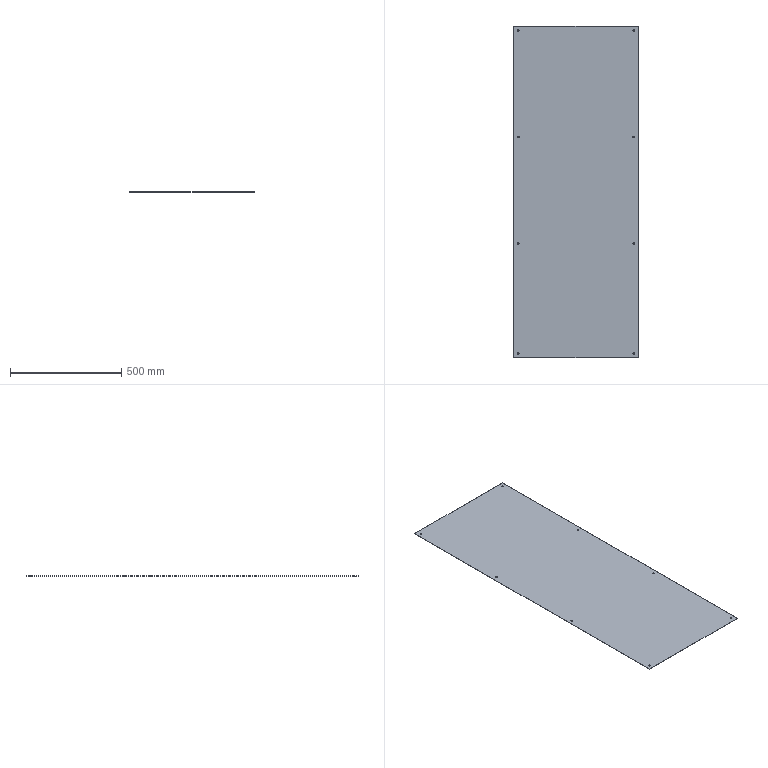Part | SolidWorks | features FlatPattern 1, HoleWzd 1, SMBaseFlange 1, SheetMetal 1 | 1 solid | 22 faces | box 560 x 1495 x 1.2 mm | volume 1004271 mm3 | cylinder 16 | plane 6 | commonest cylinder face diameters 7 x16
STEP:
#1=CARTESIAN_POINT('',(16.5,-1475.,0.));
#2=VERTEX_POINT('',#1);
#3=CARTESIAN_POINT('',(23.5,-1475.,0.));
#4=VERTEX_POINT('',#3);
#5=CARTESIAN_POINT('',(20.,-1475.,0.));
#6=DIRECTION('',(0.,0.,1.));
#7=DIRECTION('',(1.,0.,0.));
#8=AXIS2_PLACEMENT_3D('',#5,#6,#7);
#9=CIRCLE('',#8,3.5);
#10=EDGE_CURVE('',#2,#4,#9,.T.);
#11=ORIENTED_EDGE('',*,*,#10,.F.);
#12=CARTESIAN_POINT('',(16.5,-1475.,1.2));
#13=VERTEX_POINT('',#12);
#14=CARTESIAN_POINT('',(16.5,-1475.,1.2));
#15=DIRECTION('',(0.,0.,1.));
#16=VECTOR('',#15,1000.);
#17=LINE('',#14,#16);
#18=EDGE_CURVE('',#2,#13,#17,.T.);
#19=ORIENTED_EDGE('',*,*,#18,.T.);
#20=CARTESIAN_POINT('',(23.5,-1475.,1.2));
#21=VERTEX_POINT('',#20);
#22=CARTESIAN_POINT('',(20.,-1475.,1.2));
#23=DIRECTION('',(0.,0.,1.));
#24=DIRECTION('',(1.,0.,0.));
#25=AXIS2_PLACEMENT_3D('',#22,#23,#24);
#26=CIRCLE('',#25,3.5);
#27=EDGE_CURVE('',#13,#21,#26,.T.);
#28=ORIENTED_EDGE('',*,*,#27,.T.);
#29=CARTESIAN_POINT('',(23.5,-1475.,1.2));
#30=DIRECTION('',(0.,0.,1.));
#31=VECTOR('',#30,1000.);
#32=LINE('',#29,#31);
#33=EDGE_CURVE('',#4,#21,#32,.T.);
#34=ORIENTED_EDGE('',*,*,#33,.F.);
#35=EDGE_LOOP('',(#11,#19,#28,#34));
#36=FACE_OUTER_BOUND('',#35,.T.);
#37=CARTESIAN_POINT('',(20.,-1475.,1.2));
#38=DIRECTION('',(0.,0.,1.));
#39=DIRECTION('',(1.,0.,0.));
#40=AXIS2_PLACEMENT_3D('',#37,#38,#39);
#41=CYLINDRICAL_SURFACE('',#40,3.5);
#42=ADVANCED_FACE('',(#36),#41,.F.);
#43=CARTESIAN_POINT('',(536.5,-1475.,0.));
#44=VERTEX_POINT('',#43);
#45=CARTESIAN_POINT('',(543.5,-1475.,0.));
#46=VERTEX_POINT('',#45);
#47=CARTESIAN_POINT('',(540.,-1475.,0.));
#48=DIRECTION('',(0.,0.,1.));
#49=DIRECTION('',(1.,0.,0.));
#50=AXIS2_PLACEMENT_3D('',#47,#48,#49);
#51=CIRCLE('',#50,3.5);
#52=EDGE_CURVE('',#44,#46,#51,.T.);
#53=ORIENTED_EDGE('',*,*,#52,.F.);
#54=CARTESIAN_POINT('',(536.5,-1475.,1.2));
#55=VERTEX_POINT('',#54);
#56=CARTESIAN_POINT('',(536.5,-1475.,1.2));
#57=DIRECTION('',(0.,0.,1.));
#58=VECTOR('',#57,1000.);
#59=LINE('',#56,#58);
#60=EDGE_CURVE('',#44,#55,#59,.T.);
#61=ORIENTED_EDGE('',*,*,#60,.T.);
#62=CARTESIAN_POINT('',(543.5,-1475.,1.2));
#63=VERTEX_POINT('',#62);
#64=CARTESIAN_POINT('',(540.,-1475.,1.2));
#65=DIRECTION('',(0.,0.,1.));
#66=DIRECTION('',(1.,0.,0.));
#67=AXIS2_PLACEMENT_3D('',#64,#65,#66);
#68=CIRCLE('',#67,3.5);
#69=EDGE_CURVE('',#55,#63,#68,.T.);
#70=ORIENTED_EDGE('',*,*,#69,.T.);
#71=CARTESIAN_POINT('',(543.5,-1475.,1.2));
#72=DIRECTION('',(0.,0.,1.));
#73=VECTOR('',#72,1000.);
#74=LINE('',#71,#73);
#75=EDGE_CURVE('',#46,#63,#74,.T.);
#76=ORIENTED_EDGE('',*,*,#75,.F.);
#77=EDGE_LOOP('',(#53,#61,#70,#76));
#78=FACE_OUTER_BOUND('',#77,.T.);
#79=CARTESIAN_POINT('',(540.,-1475.,1.2));
#80=DIRECTION('',(0.,0.,1.));
#81=DIRECTION('',(1.,0.,0.));
#82=AXIS2_PLACEMENT_3D('',#79,#80,#81);
#83=CYLINDRICAL_SURFACE('',#82,3.5);
#84=ADVANCED_FACE('',(#78),#83,.F.);
#85=CARTESIAN_POINT('',(536.5,-500.,0.));
#86=VERTEX_POINT('',#85);
#87=CARTESIAN_POINT('',(543.5,-500.,0.));
#88=VERTEX_POINT('',#87);
#89=CARTESIAN_POINT('',(540.,-500.,0.));
#90=DIRECTION('',(0.,0.,1.));
#91=DIRECTION('',(1.,0.,0.));
#92=AXIS2_PLACEMENT_3D('',#89,#90,#91);
#93=CIRCLE('',#92,3.5);
#94=EDGE_CURVE('',#86,#88,#93,.T.);
#95=ORIENTED_EDGE('',*,*,#94,.F.);
#96=CARTESIAN_POINT('',(536.5,-500.,1.2));
#97=VERTEX_POINT('',#96);
#98=CARTESIAN_POINT('',(536.5,-500.,1.2));
#99=DIRECTION('',(0.,0.,1.));
#100=VECTOR('',#99,1000.);
#101=LINE('',#98,#100);
#102=EDGE_CURVE('',#86,#97,#101,.T.);
#103=ORIENTED_EDGE('',*,*,#102,.T.);
#104=CARTESIAN_POINT('',(543.5,-500.,1.2));
#105=VERTEX_POINT('',#104);
#106=CARTESIAN_POINT('',(540.,-500.,1.2));
#107=DIRECTION('',(0.,0.,1.));
#108=DIRECTION('',(1.,0.,0.));
#109=AXIS2_PLACEMENT_3D('',#106,#107,#108);
#110=CIRCLE('',#109,3.5);
#111=EDGE_CURVE('',#97,#105,#110,.T.);
#112=ORIENTED_EDGE('',*,*,#111,.T.);
#113=CARTESIAN_POINT('',(543.5,-500.,1.2));
#114=DIRECTION('',(0.,0.,1.));
#115=VECTOR('',#114,1000.);
#116=LINE('',#113,#115);
#117=EDGE_CURVE('',#88,#105,#116,.T.);
#118=ORIENTED_EDGE('',*,*,#117,.F.);
#119=EDGE_LOOP('',(#95,#103,#112,#118));
#120=FACE_OUTER_BOUND('',#119,.T.);
#121=CARTESIAN_POINT('',(540.,-500.,1.2));
#122=DIRECTION('',(0.,0.,1.));
#123=DIRECTION('',(1.,0.,0.));
#124=AXIS2_PLACEMENT_3D('',#121,#122,#123);
#125=CYLINDRICAL_SURFACE('',#124,3.5);
#126=ADVANCED_FACE('',(#120),#125,.F.);
#127=CARTESIAN_POINT('',(16.5,-500.,0.));
#128=VERTEX_POINT('',#127);
#129=CARTESIAN_POINT('',(23.5,-500.,0.));
#130=VERTEX_POINT('',#129);
#131=CARTESIAN_POINT('',(20.,-500.,0.));
#132=DIRECTION('',(0.,0.,1.));
#133=DIRECTION('',(1.,0.,0.));
#134=AXIS2_PLACEMENT_3D('',#131,#132,#133);
#135=CIRCLE('',#134,3.5);
#136=EDGE_CURVE('',#128,#130,#135,.T.);
#137=ORIENTED_EDGE('',*,*,#136,.F.);
#138=CARTESIAN_POINT('',(16.5,-500.,1.2));
#139=VERTEX_POINT('',#138);
#140=CARTESIAN_POINT('',(16.5,-500.,1.2));
#141=DIRECTION('',(0.,0.,1.));
#142=VECTOR('',#141,1000.);
#143=LINE('',#140,#142);
#144=EDGE_CURVE('',#128,#139,#143,.T.);
#145=ORIENTED_EDGE('',*,*,#144,.T.);
#146=CARTESIAN_POINT('',(23.5,-500.,1.2));
#147=VERTEX_POINT('',#146);
#148=CARTESIAN_POINT('',(20.,-500.,1.2));
#149=DIRECTION('',(0.,0.,1.));
#150=DIRECTION('',(1.,0.,0.));
#151=AXIS2_PLACEMENT_3D('',#148,#149,#150);
#152=CIRCLE('',#151,3.5);
#153=EDGE_CURVE('',#139,#147,#152,.T.);
#154=ORIENTED_EDGE('',*,*,#153,.T.);
#155=CARTESIAN_POINT('',(23.5,-500.,1.2));
#156=DIRECTION('',(0.,0.,1.));
#157=VECTOR('',#156,1000.);
#158=LINE('',#155,#157);
#159=EDGE_CURVE('',#130,#147,#158,.T.);
#160=ORIENTED_EDGE('',*,*,#159,.F.);
#161=EDGE_LOOP('',(#137,#145,#154,#160));
#162=FACE_OUTER_BOUND('',#161,.T.);
#163=CARTESIAN_POINT('',(20.,-500.,1.2));
#164=DIRECTION('',(0.,0.,1.));
#165=DIRECTION('',(1.,0.,0.));
#166=AXIS2_PLACEMENT_3D('',#163,#164,#165);
#167=CYLINDRICAL_SURFACE('',#166,3.5);
#168=ADVANCED_FACE('',(#162),#167,.F.);
#169=CARTESIAN_POINT('',(536.5,-20.,0.));
#170=VERTEX_POINT('',#169);
#171=CARTESIAN_POINT('',(543.5,-20.,0.));
#172=VERTEX_POINT('',#171);
#173=CARTESIAN_POINT('',(540.,-20.,0.));
#174=DIRECTION('',(0.,0.,1.));
#175=DIRECTION('',(1.,0.,0.));
#176=AXIS2_PLACEMENT_3D('',#173,#174,#175);
#177=CIRCLE('',#176,3.5);
#178=EDGE_CURVE('',#170,#172,#177,.T.);
#179=ORIENTED_EDGE('',*,*,#178,.F.);
#180=CARTESIAN_POINT('',(536.5,-20.,1.2));
#181=VERTEX_POINT('',#180);
#182=CARTESIAN_POINT('',(536.5,-20.,1.2));
#183=DIRECTION('',(0.,0.,1.));
#184=VECTOR('',#183,1000.);
#185=LINE('',#182,#184);
#186=EDGE_CURVE('',#170,#181,#185,.T.);
#187=ORIENTED_EDGE('',*,*,#186,.T.);
#188=CARTESIAN_POINT('',(543.5,-20.,1.2));
#189=VERTEX_POINT('',#188);
#190=CARTESIAN_POINT('',(540.,-20.,1.2));
#191=DIRECTION('',(0.,0.,1.));
#192=DIRECTION('',(1.,0.,0.));
#193=AXIS2_PLACEMENT_3D('',#190,#191,#192);
#194=CIRCLE('',#193,3.5);
#195=EDGE_CURVE('',#181,#189,#194,.T.);
#196=ORIENTED_EDGE('',*,*,#195,.T.);
#197=CARTESIAN_POINT('',(543.5,-20.,1.2));
#198=DIRECTION('',(0.,0.,1.));
#199=VECTOR('',#198,1000.);
#200=LINE('',#197,#199);
#201=EDGE_CURVE('',#172,#189,#200,.T.);
#202=ORIENTED_EDGE('',*,*,#201,.F.);
#203=EDGE_LOOP('',(#179,#187,#196,#202));
#204=FACE_OUTER_BOUND('',#203,.T.);
#205=CARTESIAN_POINT('',(540.,-20.,1.2));
#206=DIRECTION('',(0.,0.,1.));
#207=DIRECTION('',(1.,0.,0.));
#208=AXIS2_PLACEMENT_3D('',#205,#206,#207);
#209=CYLINDRICAL_SURFACE('',#208,3.5);
#210=ADVANCED_FACE('',(#204),#209,.F.);
#211=CARTESIAN_POINT('',(16.5,-20.,0.));
#212=VERTEX_POINT('',#211);
#213=CARTESIAN_POINT('',(23.5,-20.,0.));
#214=VERTEX_POINT('',#213);
#215=CARTESIAN_POINT('',(20.,-20.,0.));
#216=DIRECTION('',(0.,0.,1.));
#217=DIRECTION('',(1.,0.,0.));
#218=AXIS2_PLACEMENT_3D('',#215,#216,#217);
#219=CIRCLE('',#218,3.5);
#220=EDGE_CURVE('',#212,#214,#219,.T.);
#221=ORIENTED_EDGE('',*,*,#220,.F.);
#222=CARTESIAN_POINT('',(16.5,-20.,1.2));
#223=VERTEX_POINT('',#222);
#224=CARTESIAN_POINT('',(16.5,-20.,1.2));
#225=DIRECTION('',(0.,0.,1.));
#226=VECTOR('',#225,1000.);
#227=LINE('',#224,#226);
#228=EDGE_CURVE('',#212,#223,#227,.T.);
#229=ORIENTED_EDGE('',*,*,#228,.T.);
#230=CARTESIAN_POINT('',(23.5,-20.,1.2));
#231=VERTEX_POINT('',#230);
#232=CARTESIAN_POINT('',(20.,-20.,1.2));
#233=DIRECTION('',(0.,0.,1.));
#234=DIRECTION('',(1.,0.,0.));
#235=AXIS2_PLACEMENT_3D('',#232,#233,#234);
#236=CIRCLE('',#235,3.5);
#237=EDGE_CURVE('',#223,#231,#236,.T.);
#238=ORIENTED_EDGE('',*,*,#237,.T.);
#239=CARTESIAN_POINT('',(23.5,-20.,1.2));
#240=DIRECTION('',(0.,0.,1.));
#241=VECTOR('',#240,1000.);
#242=LINE('',#239,#241);
#243=EDGE_CURVE('',#214,#231,#242,.T.);
#244=ORIENTED_EDGE('',*,*,#243,.F.);
#245=EDGE_LOOP('',(#221,#229,#238,#244));
#246=FACE_OUTER_BOUND('',#245,.T.);
#247=CARTESIAN_POINT('',(20.,-20.,1.2));
#248=DIRECTION('',(0.,0.,1.));
#249=DIRECTION('',(1.,0.,0.));
#250=AXIS2_PLACEMENT_3D('',#247,#248,#249);
#251=CYLINDRICAL_SURFACE('',#250,3.5);
#252=ADVANCED_FACE('',(#246),#251,.F.);
#253=CARTESIAN_POINT('',(16.5,-980.,0.));
#254=VERTEX_POINT('',#253);
#255=CARTESIAN_POINT('',(23.5,-980.,0.));
#256=VERTEX_POINT('',#255);
#257=CARTESIAN_POINT('',(20.,-980.,0.));
#258=DIRECTION('',(0.,0.,1.));
#259=DIRECTION('',(1.,0.,0.));
#260=AXIS2_PLACEMENT_3D('',#257,#258,#259);
#261=CIRCLE('',#260,3.5);
#262=EDGE_CURVE('',#254,#256,#261,.T.);
#263=ORIENTED_EDGE('',*,*,#262,.F.);
#264=CARTESIAN_POINT('',(16.5,-980.,1.2));
#265=VERTEX_POINT('',#264);
#266=CARTESIAN_POINT('',(16.5,-980.,1.2));
#267=DIRECTION('',(0.,0.,1.));
#268=VECTOR('',#267,1000.);
#269=LINE('',#266,#268);
#270=EDGE_CURVE('',#254,#265,#269,.T.);
#271=ORIENTED_EDGE('',*,*,#270,.T.);
#272=CARTESIAN_POINT('',(23.5,-980.,1.2));
#273=VERTEX_POINT('',#272);
#274=CARTESIAN_POINT('',(20.,-980.,1.2));
#275=DIRECTION('',(0.,0.,1.));
#276=DIRECTION('',(1.,0.,0.));
#277=AXIS2_PLACEMENT_3D('',#274,#275,#276);
#278=CIRCLE('',#277,3.5);
#279=EDGE_CURVE('',#265,#273,#278,.T.);
#280=ORIENTED_EDGE('',*,*,#279,.T.);
#281=CARTESIAN_POINT('',(23.5,-980.,1.2));
#282=DIRECTION('',(0.,0.,1.));
#283=VECTOR('',#282,1000.);
#284=LINE('',#281,#283);
#285=EDGE_CURVE('',#256,#273,#284,.T.);
#286=ORIENTED_EDGE('',*,*,#285,.F.);
#287=EDGE_LOOP('',(#263,#271,#280,#286));
#288=FACE_OUTER_BOUND('',#287,.T.);
#289=CARTESIAN_POINT('',(20.,-980.,1.2));
#290=DIRECTION('',(0.,0.,1.));
#291=DIRECTION('',(1.,0.,0.));
#292=AXIS2_PLACEMENT_3D('',#289,#290,#291);
#293=CYLINDRICAL_SURFACE('',#292,3.5);
#294=ADVANCED_FACE('',(#288),#293,.F.);
#295=CARTESIAN_POINT('',(536.5,-980.,0.));
#296=VERTEX_POINT('',#295);
#297=CARTESIAN_POINT('',(543.5,-980.,0.));
#298=VERTEX_POINT('',#297);
#299=CARTESIAN_POINT('',(540.,-980.,0.));
#300=DIRECTION('',(0.,0.,1.));
#301=DIRECTION('',(1.,0.,0.));
#302=AXIS2_PLACEMENT_3D('',#299,#300,#301);
#303=CIRCLE('',#302,3.5);
#304=EDGE_CURVE('',#296,#298,#303,.T.);
#305=ORIENTED_EDGE('',*,*,#304,.F.);
#306=CARTESIAN_POINT('',(536.5,-980.,1.2));
#307=VERTEX_POINT('',#306);
#308=CARTESIAN_POINT('',(536.5,-980.,1.2));
#309=DIRECTION('',(0.,0.,1.));
#310=VECTOR('',#309,1000.);
#311=LINE('',#308,#310);
#312=EDGE_CURVE('',#296,#307,#311,.T.);
#313=ORIENTED_EDGE('',*,*,#312,.T.);
#314=CARTESIAN_POINT('',(543.5,-980.,1.2));
#315=VERTEX_POINT('',#314);
#316=CARTESIAN_POINT('',(540.,-980.,1.2));
#317=DIRECTION('',(0.,0.,1.));
#318=DIRECTION('',(1.,0.,0.));
#319=AXIS2_PLACEMENT_3D('',#316,#317,#318);
#320=CIRCLE('',#319,3.5);
#321=EDGE_CURVE('',#307,#315,#320,.T.);
#322=ORIENTED_EDGE('',*,*,#321,.T.);
#323=CARTESIAN_POINT('',(543.5,-980.,1.2));
#324=DIRECTION('',(0.,0.,1.));
#325=VECTOR('',#324,1000.);
#326=LINE('',#323,#325);
#327=EDGE_CURVE('',#298,#315,#326,.T.);
#328=ORIENTED_EDGE('',*,*,#327,.F.);
#329=EDGE_LOOP('',(#305,#313,#322,#328));
#330=FACE_OUTER_BOUND('',#329,.T.);
#331=CARTESIAN_POINT('',(540.,-980.,1.2));
#332=DIRECTION('',(0.,0.,1.));
#333=DIRECTION('',(1.,0.,0.));
#334=AXIS2_PLACEMENT_3D('',#331,#332,#333);
#335=CYLINDRICAL_SURFACE('',#334,3.5);
#336=ADVANCED_FACE('',(#330),#335,.F.);
#337=CARTESIAN_POINT('',(0.,-1495.,0.));
#338=VERTEX_POINT('',#337);
#339=CARTESIAN_POINT('',(0.,0.,0.));
#340=VERTEX_POINT('',#339);
#341=CARTESIAN_POINT('',(0.,0.,0.));
#342=DIRECTION('',(0.,1.,0.));
#343=VECTOR('',#342,1000.);
#344=LINE('',#341,#343);
#345=EDGE_CURVE('',#338,#340,#344,.T.);
#346=ORIENTED_EDGE('',*,*,#345,.F.);
#347=CARTESIAN_POINT('',(0.,-1495.,1.2));
#348=VERTEX_POINT('',#347);
#349=CARTESIAN_POINT('',(0.,-1495.,1.2));
#350=DIRECTION('',(0.,0.,-1.));
#351=VECTOR('',#350,1000.);
#352=LINE('',#349,#351);
#353=EDGE_CURVE('',#348,#338,#352,.T.);
#354=ORIENTED_EDGE('',*,*,#353,.F.);
#355=CARTESIAN_POINT('',(0.,0.,1.2));
#356=VERTEX_POINT('',#355);
#357=CARTESIAN_POINT('',(0.,0.,1.2));
#358=DIRECTION('',(0.,1.,0.));
#359=VECTOR('',#358,1000.);
#360=LINE('',#357,#359);
#361=EDGE_CURVE('',#348,#356,#360,.T.);
#362=ORIENTED_EDGE('',*,*,#361,.T.);
#363=CARTESIAN_POINT('',(0.,0.,1.2));
#364=DIRECTION('',(0.,0.,-1.));
#365=VECTOR('',#364,1000.);
#366=LINE('',#363,#365);
#367=EDGE_CURVE('',#356,#340,#366,.T.);
#368=ORIENTED_EDGE('',*,*,#367,.T.);
#369=EDGE_LOOP('',(#346,#354,#362,#368));
#370=FACE_OUTER_BOUND('',#369,.T.);
#371=CARTESIAN_POINT('',(0.,0.,1.2));
#372=DIRECTION('',(-1.,0.,0.));
#373=DIRECTION('',(0.,0.,1.));
#374=AXIS2_PLACEMENT_3D('',#371,#372,#373);
#375=PLANE('',#374);
#376=ADVANCED_FACE('',(#370),#375,.T.);
#377=CARTESIAN_POINT('',(560.,-1495.,0.));
#378=VERTEX_POINT('',#377);
#379=CARTESIAN_POINT('',(0.,-1495.,0.));
#380=DIRECTION('',(-1.,0.,0.));
#381=VECTOR('',#380,1000.);
#382=LINE('',#379,#381);
#383=EDGE_CURVE('',#378,#338,#382,.T.);
#384=ORIENTED_EDGE('',*,*,#383,.F.);
#385=CARTESIAN_POINT('',(560.,-1495.,1.2));
#386=VERTEX_POINT('',#385);
#387=CARTESIAN_POINT('',(560.,-1495.,1.2));
#388=DIRECTION('',(0.,0.,-1.));
#389=VECTOR('',#388,1000.);
#390=LINE('',#387,#389);
#391=EDGE_CURVE('',#386,#378,#390,.T.);
#392=ORIENTED_EDGE('',*,*,#391,.F.);
#393=CARTESIAN_POINT('',(0.,-1495.,1.2));
#394=DIRECTION('',(-1.,0.,0.));
#395=VECTOR('',#394,1000.);
#396=LINE('',#393,#395);
#397=EDGE_CURVE('',#386,#348,#396,.T.);
#398=ORIENTED_EDGE('',*,*,#397,.T.);
#399=ORIENTED_EDGE('',*,*,#353,.T.);
#400=EDGE_LOOP('',(#384,#392,#398,#399));
#401=FACE_OUTER_BOUND('',#400,.T.);
#402=CARTESIAN_POINT('',(0.,-1495.,1.2));
#403=DIRECTION('',(0.,-1.,0.));
#404=DIRECTION('',(0.,0.,-1.));
#405=AXIS2_PLACEMENT_3D('',#402,#403,#404);
#406=PLANE('',#405);
#407=ADVANCED_FACE('',(#401),#406,.T.);
#408=CARTESIAN_POINT('',(560.,0.,0.));
#409=VERTEX_POINT('',#408);
#410=CARTESIAN_POINT('',(560.,0.,0.));
#411=DIRECTION('',(0.,-1.,0.));
#412=VECTOR('',#411,1000.);
#413=LINE('',#410,#412);
#414=EDGE_CURVE('',#409,#378,#413,.T.);
#415=ORIENTED_EDGE('',*,*,#414,.F.);
#416=CARTESIAN_POINT('',(560.,0.,1.2));
#417=VERTEX_POINT('',#416);
#418=CARTESIAN_POINT('',(560.,0.,1.2));
#419=DIRECTION('',(0.,0.,-1.));
#420=VECTOR('',#419,1000.);
#421=LINE('',#418,#420);
#422=EDGE_CURVE('',#417,#409,#421,.T.);
#423=ORIENTED_EDGE('',*,*,#422,.F.);
#424=CARTESIAN_POINT('',(560.,0.,1.2));
#425=DIRECTION('',(0.,-1.,0.));
#426=VECTOR('',#425,1000.);
#427=LINE('',#424,#426);
#428=EDGE_CURVE('',#417,#386,#427,.T.);
#429=ORIENTED_EDGE('',*,*,#428,.T.);
#430=ORIENTED_EDGE('',*,*,#391,.T.);
#431=EDGE_LOOP('',(#415,#423,#429,#430));
#432=FACE_OUTER_BOUND('',#431,.T.);
#433=CARTESIAN_POINT('',(560.,0.,1.2));
#434=DIRECTION('',(1.,0.,0.));
#435=DIRECTION('',(0.,0.,-1.));
#436=AXIS2_PLACEMENT_3D('',#433,#434,#435);
#437=PLANE('',#436);
#438=ADVANCED_FACE('',(#432),#437,.T.);
#439=CARTESIAN_POINT('',(0.,0.,0.));
#440=DIRECTION('',(1.,0.,0.));
#441=VECTOR('',#440,1000.);
#442=LINE('',#439,#441);
#443=EDGE_CURVE('',#340,#409,#442,.T.);
#444=ORIENTED_EDGE('',*,*,#443,.F.);
#445=ORIENTED_EDGE('',*,*,#367,.F.);
#446=CARTESIAN_POINT('',(0.,0.,1.2));
#447=DIRECTION('',(1.,0.,0.));
#448=VECTOR('',#447,1000.);
#449=LINE('',#446,#448);
#450=EDGE_CURVE('',#356,#417,#449,.T.);
#451=ORIENTED_EDGE('',*,*,#450,.T.);
#452=ORIENTED_EDGE('',*,*,#422,.T.);
#453=EDGE_LOOP('',(#444,#445,#451,#452));
#454=FACE_OUTER_BOUND('',#453,.T.);
#455=CARTESIAN_POINT('',(0.,0.,1.2));
#456=DIRECTION('',(0.,1.,0.));
#457=DIRECTION('',(0.,0.,1.));
#458=AXIS2_PLACEMENT_3D('',#455,#456,#457);
#459=PLANE('',#458);
#460=ADVANCED_FACE('',(#454),#459,.T.);
#461=CARTESIAN_POINT('',(20.,-1475.,1.2));
#462=DIRECTION('',(0.,0.,1.));
#463=DIRECTION('',(1.,0.,0.));
#464=AXIS2_PLACEMENT_3D('',#461,#462,#463);
#465=CIRCLE('',#464,3.5);
#466=EDGE_CURVE('',#21,#13,#465,.T.);
#467=ORIENTED_EDGE('',*,*,#466,.F.);
#468=ORIENTED_EDGE('',*,*,#27,.F.);
#469=EDGE_LOOP('',(#467,#468));
#470=FACE_BOUND('',#469,.T.);
#471=CARTESIAN_POINT('',(540.,-1475.,1.2));
#472=DIRECTION('',(0.,0.,1.));
#473=DIRECTION('',(1.,0.,0.));
#474=AXIS2_PLACEMENT_3D('',#471,#472,#473);
#475=CIRCLE('',#474,3.5);
#476=EDGE_CURVE('',#63,#55,#475,.T.);
#477=ORIENTED_EDGE('',*,*,#476,.F.);
#478=ORIENTED_EDGE('',*,*,#69,.F.);
#479=EDGE_LOOP('',(#477,#478));
#480=FACE_BOUND('',#479,.T.);
#481=CARTESIAN_POINT('',(540.,-500.,1.2));
#482=DIRECTION('',(0.,0.,1.));
#483=DIRECTION('',(1.,0.,0.));
#484=AXIS2_PLACEMENT_3D('',#481,#482,#483);
#485=CIRCLE('',#484,3.5);
#486=EDGE_CURVE('',#105,#97,#485,.T.);
#487=ORIENTED_EDGE('',*,*,#486,.F.);
#488=ORIENTED_EDGE('',*,*,#111,.F.);
#489=EDGE_LOOP('',(#487,#488));
#490=FACE_BOUND('',#489,.T.);
#491=CARTESIAN_POINT('',(20.,-500.,1.2));
#492=DIRECTION('',(0.,0.,1.));
#493=DIRECTION('',(1.,0.,0.));
#494=AXIS2_PLACEMENT_3D('',#491,#492,#493);
#495=CIRCLE('',#494,3.5);
#496=EDGE_CURVE('',#147,#139,#495,.T.);
#497=ORIENTED_EDGE('',*,*,#496,.F.);
#498=ORIENTED_EDGE('',*,*,#153,.F.);
#499=EDGE_LOOP('',(#497,#498));
#500=FACE_BOUND('',#499,.T.);
#501=CARTESIAN_POINT('',(540.,-20.,1.2));
#502=DIRECTION('',(0.,0.,1.));
#503=DIRECTION('',(1.,0.,0.));
#504=AXIS2_PLACEMENT_3D('',#501,#502,#503);
#505=CIRCLE('',#504,3.5);
#506=EDGE_CURVE('',#189,#181,#505,.T.);
#507=ORIENTED_EDGE('',*,*,#506,.F.);
#508=ORIENTED_EDGE('',*,*,#195,.F.);
#509=EDGE_LOOP('',(#507,#508));
#510=FACE_BOUND('',#509,.T.);
#511=CARTESIAN_POINT('',(20.,-20.,1.2));
#512=DIRECTION('',(0.,0.,1.));
#513=DIRECTION('',(1.,0.,0.));
#514=AXIS2_PLACEMENT_3D('',#511,#512,#513);
#515=CIRCLE('',#514,3.5);
#516=EDGE_CURVE('',#231,#223,#515,.T.);
#517=ORIENTED_EDGE('',*,*,#516,.F.);
#518=ORIENTED_EDGE('',*,*,#237,.F.);
#519=EDGE_LOOP('',(#517,#518));
#520=FACE_BOUND('',#519,.T.);
#521=CARTESIAN_POINT('',(20.,-980.,1.2));
#522=DIRECTION('',(0.,0.,1.));
#523=DIRECTION('',(1.,0.,0.));
#524=AXIS2_PLACEMENT_3D('',#521,#522,#523);
#525=CIRCLE('',#524,3.5);
#526=EDGE_CURVE('',#273,#265,#525,.T.);
#527=ORIENTED_EDGE('',*,*,#526,.F.);
#528=ORIENTED_EDGE('',*,*,#279,.F.);
#529=EDGE_LOOP('',(#527,#528));
#530=FACE_BOUND('',#529,.T.);
#531=CARTESIAN_POINT('',(540.,-980.,1.2));
#532=DIRECTION('',(0.,0.,1.));
#533=DIRECTION('',(1.,0.,0.));
#534=AXIS2_PLACEMENT_3D('',#531,#532,#533);
#535=CIRCLE('',#534,3.5);
#536=EDGE_CURVE('',#315,#307,#535,.T.);
#537=ORIENTED_EDGE('',*,*,#536,.F.);
#538=ORIENTED_EDGE('',*,*,#321,.F.);
#539=EDGE_LOOP('',(#537,#538));
#540=FACE_BOUND('',#539,.T.);
#541=ORIENTED_EDGE('',*,*,#361,.F.);
#542=ORIENTED_EDGE('',*,*,#397,.F.);
#543=ORIENTED_EDGE('',*,*,#428,.F.);
#544=ORIENTED_EDGE('',*,*,#450,.F.);
#545=EDGE_LOOP('',(#541,#542,#543,#544));
#546=FACE_OUTER_BOUND('',#545,.T.);
#547=CARTESIAN_POINT('',(0.,0.,1.2));
#548=DIRECTION('',(0.,0.,1.));
#549=DIRECTION('',(1.,0.,0.));
#550=AXIS2_PLACEMENT_3D('',#547,#548,#549);
#551=PLANE('',#550);
#552=ADVANCED_FACE('',(#470,#480,#490,#500,#510,#520,#530,#540,#546),#551,.T.);
#553=CARTESIAN_POINT('',(20.,-1475.,0.));
#554=DIRECTION('',(0.,0.,1.));
#555=DIRECTION('',(1.,0.,0.));
#556=AXIS2_PLACEMENT_3D('',#553,#554,#555);
#557=CIRCLE('',#556,3.5);
#558=EDGE_CURVE('',#4,#2,#557,.T.);
#559=ORIENTED_EDGE('',*,*,#558,.T.);
#560=ORIENTED_EDGE('',*,*,#10,.T.);
#561=EDGE_LOOP('',(#559,#560));
#562=FACE_BOUND('',#561,.T.);
#563=CARTESIAN_POINT('',(540.,-1475.,0.));
#564=DIRECTION('',(0.,0.,1.));
#565=DIRECTION('',(1.,0.,0.));
#566=AXIS2_PLACEMENT_3D('',#563,#564,#565);
#567=CIRCLE('',#566,3.5);
#568=EDGE_CURVE('',#46,#44,#567,.T.);
#569=ORIENTED_EDGE('',*,*,#568,.T.);
#570=ORIENTED_EDGE('',*,*,#52,.T.);
#571=EDGE_LOOP('',(#569,#570));
#572=FACE_BOUND('',#571,.T.);
#573=CARTESIAN_POINT('',(540.,-500.,0.));
#574=DIRECTION('',(0.,0.,1.));
#575=DIRECTION('',(1.,0.,0.));
#576=AXIS2_PLACEMENT_3D('',#573,#574,#575);
#577=CIRCLE('',#576,3.5);
#578=EDGE_CURVE('',#88,#86,#577,.T.);
#579=ORIENTED_EDGE('',*,*,#578,.T.);
#580=ORIENTED_EDGE('',*,*,#94,.T.);
#581=EDGE_LOOP('',(#579,#580));
#582=FACE_BOUND('',#581,.T.);
#583=CARTESIAN_POINT('',(20.,-500.,0.));
#584=DIRECTION('',(0.,0.,1.));
#585=DIRECTION('',(1.,0.,0.));
#586=AXIS2_PLACEMENT_3D('',#583,#584,#585);
#587=CIRCLE('',#586,3.5);
#588=EDGE_CURVE('',#130,#128,#587,.T.);
#589=ORIENTED_EDGE('',*,*,#588,.T.);
#590=ORIENTED_EDGE('',*,*,#136,.T.);
#591=EDGE_LOOP('',(#589,#590));
#592=FACE_BOUND('',#591,.T.);
#593=CARTESIAN_POINT('',(540.,-20.,0.));
#594=DIRECTION('',(0.,0.,1.));
#595=DIRECTION('',(1.,0.,0.));
#596=AXIS2_PLACEMENT_3D('',#593,#594,#595);
#597=CIRCLE('',#596,3.5);
#598=EDGE_CURVE('',#172,#170,#597,.T.);
#599=ORIENTED_EDGE('',*,*,#598,.T.);
#600=ORIENTED_EDGE('',*,*,#178,.T.);
#601=EDGE_LOOP('',(#599,#600));
#602=FACE_BOUND('',#601,.T.);
#603=CARTESIAN_POINT('',(20.,-20.,0.));
#604=DIRECTION('',(0.,0.,1.));
#605=DIRECTION('',(1.,0.,0.));
#606=AXIS2_PLACEMENT_3D('',#603,#604,#605);
#607=CIRCLE('',#606,3.5);
#608=EDGE_CURVE('',#214,#212,#607,.T.);
#609=ORIENTED_EDGE('',*,*,#608,.T.);
#610=ORIENTED_EDGE('',*,*,#220,.T.);
#611=EDGE_LOOP('',(#609,#610));
#612=FACE_BOUND('',#611,.T.);
#613=CARTESIAN_POINT('',(20.,-980.,0.));
#614=DIRECTION('',(0.,0.,1.));
#615=DIRECTION('',(1.,0.,0.));
#616=AXIS2_PLACEMENT_3D('',#613,#614,#615);
#617=CIRCLE('',#616,3.5);
#618=EDGE_CURVE('',#256,#254,#617,.T.);
#619=ORIENTED_EDGE('',*,*,#618,.T.);
#620=ORIENTED_EDGE('',*,*,#262,.T.);
#621=EDGE_LOOP('',(#619,#620));
#622=FACE_BOUND('',#621,.T.);
#623=CARTESIAN_POINT('',(540.,-980.,0.));
#624=DIRECTION('',(0.,0.,1.));
#625=DIRECTION('',(1.,0.,0.));
#626=AXIS2_PLACEMENT_3D('',#623,#624,#625);
#627=CIRCLE('',#626,3.5);
#628=EDGE_CURVE('',#298,#296,#627,.T.);
#629=ORIENTED_EDGE('',*,*,#628,.T.);
#630=ORIENTED_EDGE('',*,*,#304,.T.);
#631=EDGE_LOOP('',(#629,#630));
#632=FACE_BOUND('',#631,.T.);
#633=ORIENTED_EDGE('',*,*,#345,.T.);
#634=ORIENTED_EDGE('',*,*,#443,.T.);
#635=ORIENTED_EDGE('',*,*,#414,.T.);
#636=ORIENTED_EDGE('',*,*,#383,.T.);
#637=EDGE_LOOP('',(#633,#634,#635,#636));
#638=FACE_OUTER_BOUND('',#637,.T.);
#639=CARTESIAN_POINT('',(0.,0.,0.));
#640=DIRECTION('',(0.,0.,1.));
#641=DIRECTION('',(1.,0.,0.));
#642=AXIS2_PLACEMENT_3D('',#639,#640,#641);
#643=PLANE('',#642);
#644=ADVANCED_FACE('',(#562,#572,#582,#592,#602,#612,#622,#632,#638),#643,.F.);
#645=ORIENTED_EDGE('',*,*,#312,.F.);
#646=ORIENTED_EDGE('',*,*,#628,.F.);
#647=ORIENTED_EDGE('',*,*,#327,.T.);
#648=ORIENTED_EDGE('',*,*,#536,.T.);
#649=EDGE_LOOP('',(#645,#646,#647,#648));
#650=FACE_OUTER_BOUND('',#649,.T.);
#651=CARTESIAN_POINT('',(540.,-980.,1.2));
#652=DIRECTION('',(0.,0.,1.));
#653=DIRECTION('',(1.,0.,0.));
#654=AXIS2_PLACEMENT_3D('',#651,#652,#653);
#655=CYLINDRICAL_SURFACE('',#654,3.5);
#656=ADVANCED_FACE('',(#650),#655,.F.);
#657=ORIENTED_EDGE('',*,*,#270,.F.);
#658=ORIENTED_EDGE('',*,*,#618,.F.);
#659=ORIENTED_EDGE('',*,*,#285,.T.);
#660=ORIENTED_EDGE('',*,*,#526,.T.);
#661=EDGE_LOOP('',(#657,#658,#659,#660));
#662=FACE_OUTER_BOUND('',#661,.T.);
#663=CARTESIAN_POINT('',(20.,-980.,1.2));
#664=DIRECTION('',(0.,0.,1.));
#665=DIRECTION('',(1.,0.,0.));
#666=AXIS2_PLACEMENT_3D('',#663,#664,#665);
#667=CYLINDRICAL_SURFACE('',#666,3.5);
#668=ADVANCED_FACE('',(#662),#667,.F.);
#669=ORIENTED_EDGE('',*,*,#228,.F.);
#670=ORIENTED_EDGE('',*,*,#608,.F.);
#671=ORIENTED_EDGE('',*,*,#243,.T.);
#672=ORIENTED_EDGE('',*,*,#516,.T.);
#673=EDGE_LOOP('',(#669,#670,#671,#672));
#674=FACE_OUTER_BOUND('',#673,.T.);
#675=CARTESIAN_POINT('',(20.,-20.,1.2));
#676=DIRECTION('',(0.,0.,1.));
#677=DIRECTION('',(1.,0.,0.));
#678=AXIS2_PLACEMENT_3D('',#675,#676,#677);
#679=CYLINDRICAL_SURFACE('',#678,3.5);
#680=ADVANCED_FACE('',(#674),#679,.F.);
#681=ORIENTED_EDGE('',*,*,#186,.F.);
#682=ORIENTED_EDGE('',*,*,#598,.F.);
#683=ORIENTED_EDGE('',*,*,#201,.T.);
#684=ORIENTED_EDGE('',*,*,#506,.T.);
#685=EDGE_LOOP('',(#681,#682,#683,#684));
#686=FACE_OUTER_BOUND('',#685,.T.);
#687=CARTESIAN_POINT('',(540.,-20.,1.2));
#688=DIRECTION('',(0.,0.,1.));
#689=DIRECTION('',(1.,0.,0.));
#690=AXIS2_PLACEMENT_3D('',#687,#688,#689);
#691=CYLINDRICAL_SURFACE('',#690,3.5);
#692=ADVANCED_FACE('',(#686),#691,.F.);
#693=ORIENTED_EDGE('',*,*,#144,.F.);
#694=ORIENTED_EDGE('',*,*,#588,.F.);
#695=ORIENTED_EDGE('',*,*,#159,.T.);
#696=ORIENTED_EDGE('',*,*,#496,.T.);
#697=EDGE_LOOP('',(#693,#694,#695,#696));
#698=FACE_OUTER_BOUND('',#697,.T.);
#699=CARTESIAN_POINT('',(20.,-500.,1.2));
#700=DIRECTION('',(0.,0.,1.));
#701=DIRECTION('',(1.,0.,0.));
#702=AXIS2_PLACEMENT_3D('',#699,#700,#701);
#703=CYLINDRICAL_SURFACE('',#702,3.5);
#704=ADVANCED_FACE('',(#698),#703,.F.);
#705=ORIENTED_EDGE('',*,*,#102,.F.);
#706=ORIENTED_EDGE('',*,*,#578,.F.);
#707=ORIENTED_EDGE('',*,*,#117,.T.);
#708=ORIENTED_EDGE('',*,*,#486,.T.);
#709=EDGE_LOOP('',(#705,#706,#707,#708));
#710=FACE_OUTER_BOUND('',#709,.T.);
#711=CARTESIAN_POINT('',(540.,-500.,1.2));
#712=DIRECTION('',(0.,0.,1.));
#713=DIRECTION('',(1.,0.,0.));
#714=AXIS2_PLACEMENT_3D('',#711,#712,#713);
#715=CYLINDRICAL_SURFACE('',#714,3.5);
#716=ADVANCED_FACE('',(#710),#715,.F.);
#717=ORIENTED_EDGE('',*,*,#60,.F.);
#718=ORIENTED_EDGE('',*,*,#568,.F.);
#719=ORIENTED_EDGE('',*,*,#75,.T.);
#720=ORIENTED_EDGE('',*,*,#476,.T.);
#721=EDGE_LOOP('',(#717,#718,#719,#720));
#722=FACE_OUTER_BOUND('',#721,.T.);
#723=CARTESIAN_POINT('',(540.,-1475.,1.2));
#724=DIRECTION('',(0.,0.,1.));
#725=DIRECTION('',(1.,0.,0.));
#726=AXIS2_PLACEMENT_3D('',#723,#724,#725);
#727=CYLINDRICAL_SURFACE('',#726,3.5);
#728=ADVANCED_FACE('',(#722),#727,.F.);
#729=ORIENTED_EDGE('',*,*,#18,.F.);
#730=ORIENTED_EDGE('',*,*,#558,.F.);
#731=ORIENTED_EDGE('',*,*,#33,.T.);
#732=ORIENTED_EDGE('',*,*,#466,.T.);
#733=EDGE_LOOP('',(#729,#730,#731,#732));
#734=FACE_OUTER_BOUND('',#733,.T.);
#735=CARTESIAN_POINT('',(20.,-1475.,1.2));
#736=DIRECTION('',(0.,0.,1.));
#737=DIRECTION('',(1.,0.,0.));
#738=AXIS2_PLACEMENT_3D('',#735,#736,#737);
#739=CYLINDRICAL_SURFACE('',#738,3.5);
#740=ADVANCED_FACE('',(#734),#739,.F.);
#741=CLOSED_SHELL('',(#42,#84,#126,#168,#210,#252,#294,#336,#376,#407,#438,#460,#552,#644,#656,#668,#680,#692,#704,#716,#728,#740));
#742=MANIFOLD_SOLID_BREP('',#741);
#743=CARTESIAN_POINT('',(0.,0.,0.));
#744=DIRECTION('',(0.,0.,1.));
#745=DIRECTION('',(1.,0.,0.));
#746=AXIS2_PLACEMENT_3D('',#743,#744,#745);
#747=(LENGTH_UNIT()NAMED_UNIT(*)SI_UNIT(.MILLI.,.METRE.));
#748=UNCERTAINTY_MEASURE_WITH_UNIT(LENGTH_MEASURE(0.00001),#747,'','');
#749=(NAMED_UNIT(*)PLANE_ANGLE_UNIT()SI_UNIT($,.RADIAN.));
#750=(NAMED_UNIT(*)SI_UNIT($,.STERADIAN.)SOLID_ANGLE_UNIT());
#751=(GEOMETRIC_REPRESENTATION_CONTEXT(3)GLOBAL_UNCERTAINTY_ASSIGNED_CONTEXT((#748))GLOBAL_UNIT_ASSIGNED_CONTEXT((#747,#749,#750))REPRESENTATION_CONTEXT('',''));
#752=ADVANCED_BREP_SHAPE_REPRESENTATION('',(#742,#746),#751);